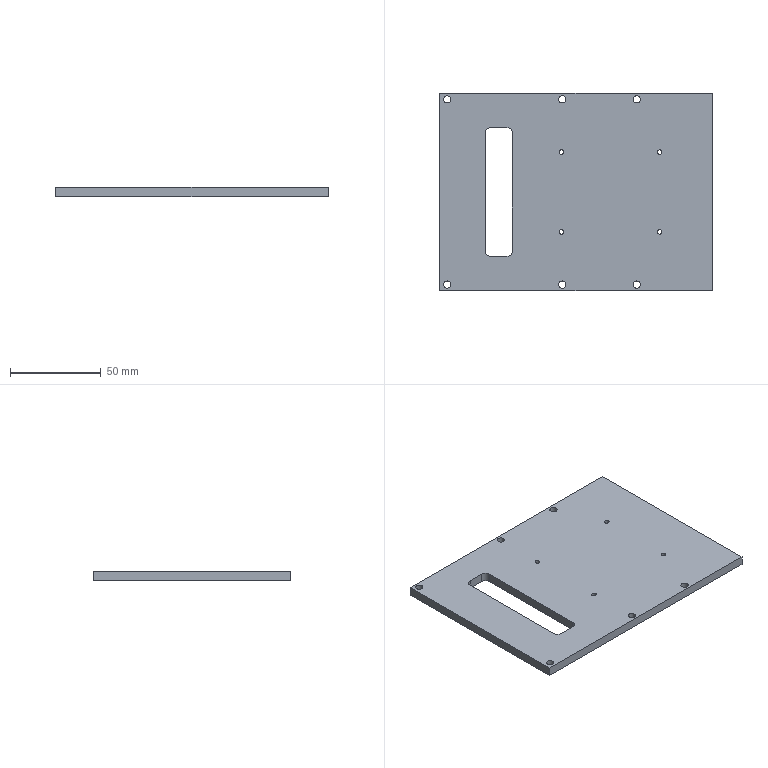Part | NX | 1 solid | 24 faces | box 150 x 108.5 x 5 mm | volume 75613 mm3 | cylinder 14 | plane 10 | commonest cylinder face diameters 4 x6 2.5 x4 6 x4
STEP:
#1=CARTESIAN_POINT('',(-38.,35.5,0.));
#2=VERTEX_POINT('',#1);
#3=CARTESIAN_POINT('',(-47.,35.5,0.));
#4=VERTEX_POINT('',#3);
#5=CARTESIAN_POINT('',(-38.,35.5,0.));
#6=DIRECTION('',(-1.,0.,0.));
#7=VECTOR('',#6,1000.);
#8=LINE('',#5,#7);
#9=EDGE_CURVE('',#2,#4,#8,.T.);
#10=ORIENTED_EDGE('',*,*,#9,.T.);
#11=CARTESIAN_POINT('',(-47.,35.5,-5.));
#12=VERTEX_POINT('',#11);
#13=CARTESIAN_POINT('',(-47.,35.5,-5.));
#14=DIRECTION('',(0.,0.,1.));
#15=VECTOR('',#14,1000.);
#16=LINE('',#13,#15);
#17=EDGE_CURVE('',#12,#4,#16,.T.);
#18=ORIENTED_EDGE('',*,*,#17,.F.);
#19=CARTESIAN_POINT('',(-38.,35.5,-5.));
#20=VERTEX_POINT('',#19);
#21=CARTESIAN_POINT('',(-38.,35.5,-5.));
#22=DIRECTION('',(-1.,0.,0.));
#23=VECTOR('',#22,1000.);
#24=LINE('',#21,#23);
#25=EDGE_CURVE('',#20,#12,#24,.T.);
#26=ORIENTED_EDGE('',*,*,#25,.F.);
#27=CARTESIAN_POINT('',(-38.,35.5,-5.));
#28=DIRECTION('',(0.,0.,1.));
#29=VECTOR('',#28,1000.);
#30=LINE('',#27,#29);
#31=EDGE_CURVE('',#20,#2,#30,.T.);
#32=ORIENTED_EDGE('',*,*,#31,.T.);
#33=EDGE_LOOP('',(#10,#18,#26,#32));
#34=FACE_BOUND('',#33,.T.);
#35=CARTESIAN_POINT('',(-38.,35.5,-5.));
#36=DIRECTION('',(0.,1.,0.));
#37=DIRECTION('',(-1.,0.,0.));
#38=AXIS2_PLACEMENT_3D('',#35,#36,#37);
#39=PLANE('',#38);
#40=ADVANCED_FACE('',(#34),#39,.F.);
#41=CARTESIAN_POINT('',(-35.,32.5,0.));
#42=VERTEX_POINT('',#41);
#43=CARTESIAN_POINT('',(-38.,32.5,0.));
#44=DIRECTION('',(0.,0.,1.));
#45=DIRECTION('',(0.,-1.,0.));
#46=AXIS2_PLACEMENT_3D('',#43,#44,#45);
#47=CIRCLE('',#46,3.);
#48=EDGE_CURVE('',#42,#2,#47,.T.);
#49=ORIENTED_EDGE('',*,*,#48,.T.);
#50=ORIENTED_EDGE('',*,*,#31,.F.);
#51=CARTESIAN_POINT('',(-35.,32.5,-5.));
#52=VERTEX_POINT('',#51);
#53=CARTESIAN_POINT('',(-38.,32.5,-5.));
#54=DIRECTION('',(0.,0.,1.));
#55=DIRECTION('',(0.,-1.,0.));
#56=AXIS2_PLACEMENT_3D('',#53,#54,#55);
#57=CIRCLE('',#56,3.);
#58=EDGE_CURVE('',#52,#20,#57,.T.);
#59=ORIENTED_EDGE('',*,*,#58,.F.);
#60=CARTESIAN_POINT('',(-35.,32.5,-5.));
#61=DIRECTION('',(0.,0.,1.));
#62=VECTOR('',#61,1000.);
#63=LINE('',#60,#62);
#64=EDGE_CURVE('',#52,#42,#63,.T.);
#65=ORIENTED_EDGE('',*,*,#64,.T.);
#66=EDGE_LOOP('',(#49,#50,#59,#65));
#67=FACE_BOUND('',#66,.T.);
#68=CARTESIAN_POINT('',(-38.,32.5,-5.));
#69=DIRECTION('',(0.,0.,1.));
#70=DIRECTION('',(0.,-1.,0.));
#71=AXIS2_PLACEMENT_3D('',#68,#69,#70);
#72=CYLINDRICAL_SURFACE('',#71,3.);
#73=ADVANCED_FACE('',(#67),#72,.F.);
#74=CARTESIAN_POINT('',(-35.,-32.5,0.));
#75=VERTEX_POINT('',#74);
#76=CARTESIAN_POINT('',(-35.,-32.5,0.));
#77=DIRECTION('',(0.,1.,0.));
#78=VECTOR('',#77,1000.);
#79=LINE('',#76,#78);
#80=EDGE_CURVE('',#75,#42,#79,.T.);
#81=ORIENTED_EDGE('',*,*,#80,.T.);
#82=ORIENTED_EDGE('',*,*,#64,.F.);
#83=CARTESIAN_POINT('',(-35.,-32.5,-5.));
#84=VERTEX_POINT('',#83);
#85=CARTESIAN_POINT('',(-35.,-32.5,-5.));
#86=DIRECTION('',(0.,1.,0.));
#87=VECTOR('',#86,1000.);
#88=LINE('',#85,#87);
#89=EDGE_CURVE('',#84,#52,#88,.T.);
#90=ORIENTED_EDGE('',*,*,#89,.F.);
#91=CARTESIAN_POINT('',(-35.,-32.5,-5.));
#92=DIRECTION('',(0.,0.,1.));
#93=VECTOR('',#92,1000.);
#94=LINE('',#91,#93);
#95=EDGE_CURVE('',#84,#75,#94,.T.);
#96=ORIENTED_EDGE('',*,*,#95,.T.);
#97=EDGE_LOOP('',(#81,#82,#90,#96));
#98=FACE_BOUND('',#97,.T.);
#99=CARTESIAN_POINT('',(-35.,-32.5,-5.));
#100=DIRECTION('',(1.,0.,0.));
#101=DIRECTION('',(0.,1.,0.));
#102=AXIS2_PLACEMENT_3D('',#99,#100,#101);
#103=PLANE('',#102);
#104=ADVANCED_FACE('',(#98),#103,.F.);
#105=CARTESIAN_POINT('',(-38.,-35.5,0.));
#106=VERTEX_POINT('',#105);
#107=CARTESIAN_POINT('',(-38.,-32.5,0.));
#108=DIRECTION('',(0.,0.,1.));
#109=DIRECTION('',(0.,-1.,0.));
#110=AXIS2_PLACEMENT_3D('',#107,#108,#109);
#111=CIRCLE('',#110,3.);
#112=EDGE_CURVE('',#106,#75,#111,.T.);
#113=ORIENTED_EDGE('',*,*,#112,.T.);
#114=ORIENTED_EDGE('',*,*,#95,.F.);
#115=CARTESIAN_POINT('',(-38.,-35.5,-5.));
#116=VERTEX_POINT('',#115);
#117=CARTESIAN_POINT('',(-38.,-32.5,-5.));
#118=DIRECTION('',(0.,0.,1.));
#119=DIRECTION('',(0.,-1.,0.));
#120=AXIS2_PLACEMENT_3D('',#117,#118,#119);
#121=CIRCLE('',#120,3.);
#122=EDGE_CURVE('',#116,#84,#121,.T.);
#123=ORIENTED_EDGE('',*,*,#122,.F.);
#124=CARTESIAN_POINT('',(-38.,-35.5,-5.));
#125=DIRECTION('',(0.,0.,1.));
#126=VECTOR('',#125,1000.);
#127=LINE('',#124,#126);
#128=EDGE_CURVE('',#116,#106,#127,.T.);
#129=ORIENTED_EDGE('',*,*,#128,.T.);
#130=EDGE_LOOP('',(#113,#114,#123,#129));
#131=FACE_BOUND('',#130,.T.);
#132=CARTESIAN_POINT('',(-38.,-32.5,-5.));
#133=DIRECTION('',(0.,0.,1.));
#134=DIRECTION('',(0.,-1.,0.));
#135=AXIS2_PLACEMENT_3D('',#132,#133,#134);
#136=CYLINDRICAL_SURFACE('',#135,3.);
#137=ADVANCED_FACE('',(#131),#136,.F.);
#138=CARTESIAN_POINT('',(-47.,-35.5,0.));
#139=VERTEX_POINT('',#138);
#140=CARTESIAN_POINT('',(-47.,-35.5,0.));
#141=DIRECTION('',(1.,0.,0.));
#142=VECTOR('',#141,1000.);
#143=LINE('',#140,#142);
#144=EDGE_CURVE('',#139,#106,#143,.T.);
#145=ORIENTED_EDGE('',*,*,#144,.T.);
#146=ORIENTED_EDGE('',*,*,#128,.F.);
#147=CARTESIAN_POINT('',(-47.,-35.5,-5.));
#148=VERTEX_POINT('',#147);
#149=CARTESIAN_POINT('',(-47.,-35.5,-5.));
#150=DIRECTION('',(1.,0.,0.));
#151=VECTOR('',#150,1000.);
#152=LINE('',#149,#151);
#153=EDGE_CURVE('',#148,#116,#152,.T.);
#154=ORIENTED_EDGE('',*,*,#153,.F.);
#155=CARTESIAN_POINT('',(-47.,-35.5,-5.));
#156=DIRECTION('',(0.,0.,1.));
#157=VECTOR('',#156,1000.);
#158=LINE('',#155,#157);
#159=EDGE_CURVE('',#148,#139,#158,.T.);
#160=ORIENTED_EDGE('',*,*,#159,.T.);
#161=EDGE_LOOP('',(#145,#146,#154,#160));
#162=FACE_BOUND('',#161,.T.);
#163=CARTESIAN_POINT('',(-47.,-35.5,-5.));
#164=DIRECTION('',(0.,-1.,0.));
#165=DIRECTION('',(0.,0.,-1.));
#166=AXIS2_PLACEMENT_3D('',#163,#164,#165);
#167=PLANE('',#166);
#168=ADVANCED_FACE('',(#162),#167,.F.);
#169=CARTESIAN_POINT('',(-50.,-32.5,0.));
#170=VERTEX_POINT('',#169);
#171=CARTESIAN_POINT('',(-47.,-32.5,0.));
#172=DIRECTION('',(0.,0.,1.));
#173=DIRECTION('',(0.,-1.,0.));
#174=AXIS2_PLACEMENT_3D('',#171,#172,#173);
#175=CIRCLE('',#174,3.);
#176=EDGE_CURVE('',#170,#139,#175,.T.);
#177=ORIENTED_EDGE('',*,*,#176,.T.);
#178=ORIENTED_EDGE('',*,*,#159,.F.);
#179=CARTESIAN_POINT('',(-50.,-32.5,-5.));
#180=VERTEX_POINT('',#179);
#181=CARTESIAN_POINT('',(-47.,-32.5,-5.));
#182=DIRECTION('',(0.,0.,1.));
#183=DIRECTION('',(0.,-1.,0.));
#184=AXIS2_PLACEMENT_3D('',#181,#182,#183);
#185=CIRCLE('',#184,3.);
#186=EDGE_CURVE('',#180,#148,#185,.T.);
#187=ORIENTED_EDGE('',*,*,#186,.F.);
#188=CARTESIAN_POINT('',(-50.,-32.5,-5.));
#189=DIRECTION('',(0.,0.,1.));
#190=VECTOR('',#189,1000.);
#191=LINE('',#188,#190);
#192=EDGE_CURVE('',#180,#170,#191,.T.);
#193=ORIENTED_EDGE('',*,*,#192,.T.);
#194=EDGE_LOOP('',(#177,#178,#187,#193));
#195=FACE_BOUND('',#194,.T.);
#196=CARTESIAN_POINT('',(-47.,-32.5,-5.));
#197=DIRECTION('',(0.,0.,1.));
#198=DIRECTION('',(0.,-1.,0.));
#199=AXIS2_PLACEMENT_3D('',#196,#197,#198);
#200=CYLINDRICAL_SURFACE('',#199,3.);
#201=ADVANCED_FACE('',(#195),#200,.F.);
#202=CARTESIAN_POINT('',(-50.,32.5,0.));
#203=VERTEX_POINT('',#202);
#204=CARTESIAN_POINT('',(-50.,32.5,0.));
#205=DIRECTION('',(0.,-1.,0.));
#206=VECTOR('',#205,1000.);
#207=LINE('',#204,#206);
#208=EDGE_CURVE('',#203,#170,#207,.T.);
#209=ORIENTED_EDGE('',*,*,#208,.T.);
#210=ORIENTED_EDGE('',*,*,#192,.F.);
#211=CARTESIAN_POINT('',(-50.,32.5,-5.));
#212=VERTEX_POINT('',#211);
#213=CARTESIAN_POINT('',(-50.,32.5,-5.));
#214=DIRECTION('',(0.,-1.,0.));
#215=VECTOR('',#214,1000.);
#216=LINE('',#213,#215);
#217=EDGE_CURVE('',#212,#180,#216,.T.);
#218=ORIENTED_EDGE('',*,*,#217,.F.);
#219=CARTESIAN_POINT('',(-50.,32.5,-5.));
#220=DIRECTION('',(0.,0.,1.));
#221=VECTOR('',#220,1000.);
#222=LINE('',#219,#221);
#223=EDGE_CURVE('',#212,#203,#222,.T.);
#224=ORIENTED_EDGE('',*,*,#223,.T.);
#225=EDGE_LOOP('',(#209,#210,#218,#224));
#226=FACE_BOUND('',#225,.T.);
#227=CARTESIAN_POINT('',(-50.,32.5,-5.));
#228=DIRECTION('',(-1.,0.,0.));
#229=DIRECTION('',(0.,0.,-1.));
#230=AXIS2_PLACEMENT_3D('',#227,#228,#229);
#231=PLANE('',#230);
#232=ADVANCED_FACE('',(#226),#231,.F.);
#233=CARTESIAN_POINT('',(75.,-54.25,0.));
#234=VERTEX_POINT('',#233);
#235=CARTESIAN_POINT('',(75.,54.25,0.));
#236=VERTEX_POINT('',#235);
#237=CARTESIAN_POINT('',(75.,-54.25,0.));
#238=DIRECTION('',(0.,1.,0.));
#239=VECTOR('',#238,1000.);
#240=LINE('',#237,#239);
#241=EDGE_CURVE('',#234,#236,#240,.T.);
#242=ORIENTED_EDGE('',*,*,#241,.F.);
#243=CARTESIAN_POINT('',(75.,-54.25,-5.));
#244=VERTEX_POINT('',#243);
#245=CARTESIAN_POINT('',(75.,-54.25,-5.));
#246=DIRECTION('',(0.,0.,1.));
#247=VECTOR('',#246,1000.);
#248=LINE('',#245,#247);
#249=EDGE_CURVE('',#244,#234,#248,.T.);
#250=ORIENTED_EDGE('',*,*,#249,.F.);
#251=CARTESIAN_POINT('',(75.,54.25,-5.));
#252=VERTEX_POINT('',#251);
#253=CARTESIAN_POINT('',(75.,-54.25,-5.));
#254=DIRECTION('',(0.,1.,0.));
#255=VECTOR('',#254,1000.);
#256=LINE('',#253,#255);
#257=EDGE_CURVE('',#244,#252,#256,.T.);
#258=ORIENTED_EDGE('',*,*,#257,.T.);
#259=CARTESIAN_POINT('',(75.,54.25,-5.));
#260=DIRECTION('',(0.,0.,1.));
#261=VECTOR('',#260,1000.);
#262=LINE('',#259,#261);
#263=EDGE_CURVE('',#252,#236,#262,.T.);
#264=ORIENTED_EDGE('',*,*,#263,.T.);
#265=EDGE_LOOP('',(#242,#250,#258,#264));
#266=FACE_BOUND('',#265,.T.);
#267=CARTESIAN_POINT('',(75.,-54.25,-5.));
#268=DIRECTION('',(1.,0.,0.));
#269=DIRECTION('',(0.,0.,1.));
#270=AXIS2_PLACEMENT_3D('',#267,#268,#269);
#271=PLANE('',#270);
#272=ADVANCED_FACE('',(#266),#271,.T.);
#273=CARTESIAN_POINT('',(-75.,54.25,0.));
#274=VERTEX_POINT('',#273);
#275=CARTESIAN_POINT('',(75.,54.25,0.));
#276=DIRECTION('',(-1.,0.,0.));
#277=VECTOR('',#276,1000.);
#278=LINE('',#275,#277);
#279=EDGE_CURVE('',#236,#274,#278,.T.);
#280=ORIENTED_EDGE('',*,*,#279,.F.);
#281=ORIENTED_EDGE('',*,*,#263,.F.);
#282=CARTESIAN_POINT('',(-75.,54.25,-5.));
#283=VERTEX_POINT('',#282);
#284=CARTESIAN_POINT('',(75.,54.25,-5.));
#285=DIRECTION('',(-1.,0.,0.));
#286=VECTOR('',#285,1000.);
#287=LINE('',#284,#286);
#288=EDGE_CURVE('',#252,#283,#287,.T.);
#289=ORIENTED_EDGE('',*,*,#288,.T.);
#290=CARTESIAN_POINT('',(-75.,54.25,-5.));
#291=DIRECTION('',(0.,0.,1.));
#292=VECTOR('',#291,1000.);
#293=LINE('',#290,#292);
#294=EDGE_CURVE('',#283,#274,#293,.T.);
#295=ORIENTED_EDGE('',*,*,#294,.T.);
#296=EDGE_LOOP('',(#280,#281,#289,#295));
#297=FACE_BOUND('',#296,.T.);
#298=CARTESIAN_POINT('',(75.,54.25,-5.));
#299=DIRECTION('',(0.,1.,0.));
#300=DIRECTION('',(0.,0.,1.));
#301=AXIS2_PLACEMENT_3D('',#298,#299,#300);
#302=PLANE('',#301);
#303=ADVANCED_FACE('',(#297),#302,.T.);
#304=CARTESIAN_POINT('',(-75.,-54.25,0.));
#305=VERTEX_POINT('',#304);
#306=CARTESIAN_POINT('',(-75.,54.25,0.));
#307=DIRECTION('',(0.,-1.,0.));
#308=VECTOR('',#307,1000.);
#309=LINE('',#306,#308);
#310=EDGE_CURVE('',#274,#305,#309,.T.);
#311=ORIENTED_EDGE('',*,*,#310,.F.);
#312=ORIENTED_EDGE('',*,*,#294,.F.);
#313=CARTESIAN_POINT('',(-75.,-54.25,-5.));
#314=VERTEX_POINT('',#313);
#315=CARTESIAN_POINT('',(-75.,54.25,-5.));
#316=DIRECTION('',(0.,-1.,0.));
#317=VECTOR('',#316,1000.);
#318=LINE('',#315,#317);
#319=EDGE_CURVE('',#283,#314,#318,.T.);
#320=ORIENTED_EDGE('',*,*,#319,.T.);
#321=CARTESIAN_POINT('',(-75.,-54.25,-5.));
#322=DIRECTION('',(0.,0.,1.));
#323=VECTOR('',#322,1000.);
#324=LINE('',#321,#323);
#325=EDGE_CURVE('',#314,#305,#324,.T.);
#326=ORIENTED_EDGE('',*,*,#325,.T.);
#327=EDGE_LOOP('',(#311,#312,#320,#326));
#328=FACE_BOUND('',#327,.T.);
#329=CARTESIAN_POINT('',(-75.,54.25,-5.));
#330=DIRECTION('',(-1.,0.,0.));
#331=DIRECTION('',(0.,0.,-1.));
#332=AXIS2_PLACEMENT_3D('',#329,#330,#331);
#333=PLANE('',#332);
#334=ADVANCED_FACE('',(#328),#333,.T.);
#335=CARTESIAN_POINT('',(-7.5,-53.,-5.));
#336=VERTEX_POINT('',#335);
#337=CARTESIAN_POINT('',(-7.5,-51.,-5.));
#338=DIRECTION('',(0.,0.,1.));
#339=DIRECTION('',(0.,-1.,0.));
#340=AXIS2_PLACEMENT_3D('',#337,#338,#339);
#341=CIRCLE('',#340,2.);
#342=EDGE_CURVE('',#336,#336,#341,.T.);
#343=ORIENTED_EDGE('',*,*,#342,.F.);
#344=EDGE_LOOP('',(#343));
#345=FACE_BOUND('',#344,.T.);
#346=CARTESIAN_POINT('',(-7.5,-53.,0.));
#347=VERTEX_POINT('',#346);
#348=CARTESIAN_POINT('',(-7.5,-51.,0.));
#349=DIRECTION('',(0.,0.,1.));
#350=DIRECTION('',(0.,-1.,0.));
#351=AXIS2_PLACEMENT_3D('',#348,#349,#350);
#352=CIRCLE('',#351,2.);
#353=EDGE_CURVE('',#347,#347,#352,.T.);
#354=ORIENTED_EDGE('',*,*,#353,.T.);
#355=EDGE_LOOP('',(#354));
#356=FACE_BOUND('',#355,.T.);
#357=CARTESIAN_POINT('',(-7.5,-51.,-5.));
#358=DIRECTION('',(0.,0.,1.));
#359=DIRECTION('',(0.,-1.,0.));
#360=AXIS2_PLACEMENT_3D('',#357,#358,#359);
#361=CYLINDRICAL_SURFACE('',#360,2.);
#362=ADVANCED_FACE('',(#345,#356),#361,.F.);
#363=CARTESIAN_POINT('',(-71.,-53.,-5.));
#364=VERTEX_POINT('',#363);
#365=CARTESIAN_POINT('',(-71.,-51.,-5.));
#366=DIRECTION('',(0.,0.,1.));
#367=DIRECTION('',(0.,-1.,0.));
#368=AXIS2_PLACEMENT_3D('',#365,#366,#367);
#369=CIRCLE('',#368,2.);
#370=EDGE_CURVE('',#364,#364,#369,.T.);
#371=ORIENTED_EDGE('',*,*,#370,.F.);
#372=EDGE_LOOP('',(#371));
#373=FACE_BOUND('',#372,.T.);
#374=CARTESIAN_POINT('',(-71.,-53.,0.));
#375=VERTEX_POINT('',#374);
#376=CARTESIAN_POINT('',(-71.,-51.,0.));
#377=DIRECTION('',(0.,0.,1.));
#378=DIRECTION('',(0.,-1.,0.));
#379=AXIS2_PLACEMENT_3D('',#376,#377,#378);
#380=CIRCLE('',#379,2.);
#381=EDGE_CURVE('',#375,#375,#380,.T.);
#382=ORIENTED_EDGE('',*,*,#381,.T.);
#383=EDGE_LOOP('',(#382));
#384=FACE_BOUND('',#383,.T.);
#385=CARTESIAN_POINT('',(-71.,-51.,-5.));
#386=DIRECTION('',(0.,0.,1.));
#387=DIRECTION('',(0.,-1.,0.));
#388=AXIS2_PLACEMENT_3D('',#385,#386,#387);
#389=CYLINDRICAL_SURFACE('',#388,2.);
#390=ADVANCED_FACE('',(#373,#384),#389,.F.);
#391=CARTESIAN_POINT('',(46.,-23.25,-5.));
#392=VERTEX_POINT('',#391);
#393=CARTESIAN_POINT('',(46.,-22.,-5.));
#394=DIRECTION('',(0.,0.,1.));
#395=DIRECTION('',(0.,-1.,0.));
#396=AXIS2_PLACEMENT_3D('',#393,#394,#395);
#397=CIRCLE('',#396,1.25);
#398=EDGE_CURVE('',#392,#392,#397,.T.);
#399=ORIENTED_EDGE('',*,*,#398,.F.);
#400=EDGE_LOOP('',(#399));
#401=FACE_BOUND('',#400,.T.);
#402=CARTESIAN_POINT('',(46.,-23.25,0.));
#403=VERTEX_POINT('',#402);
#404=CARTESIAN_POINT('',(46.,-22.,0.));
#405=DIRECTION('',(0.,0.,1.));
#406=DIRECTION('',(0.,-1.,0.));
#407=AXIS2_PLACEMENT_3D('',#404,#405,#406);
#408=CIRCLE('',#407,1.25);
#409=EDGE_CURVE('',#403,#403,#408,.T.);
#410=ORIENTED_EDGE('',*,*,#409,.T.);
#411=EDGE_LOOP('',(#410));
#412=FACE_BOUND('',#411,.T.);
#413=CARTESIAN_POINT('',(46.,-22.,-5.));
#414=DIRECTION('',(0.,0.,1.));
#415=DIRECTION('',(0.,-1.,0.));
#416=AXIS2_PLACEMENT_3D('',#413,#414,#415);
#417=CYLINDRICAL_SURFACE('',#416,1.25);
#418=ADVANCED_FACE('',(#401,#412),#417,.F.);
#419=CARTESIAN_POINT('',(-8.,-23.25,-5.));
#420=VERTEX_POINT('',#419);
#421=CARTESIAN_POINT('',(-8.,-22.,-5.));
#422=DIRECTION('',(0.,0.,1.));
#423=DIRECTION('',(0.,-1.,0.));
#424=AXIS2_PLACEMENT_3D('',#421,#422,#423);
#425=CIRCLE('',#424,1.25);
#426=EDGE_CURVE('',#420,#420,#425,.T.);
#427=ORIENTED_EDGE('',*,*,#426,.F.);
#428=EDGE_LOOP('',(#427));
#429=FACE_BOUND('',#428,.T.);
#430=CARTESIAN_POINT('',(-8.,-23.25,0.));
#431=VERTEX_POINT('',#430);
#432=CARTESIAN_POINT('',(-8.,-22.,0.));
#433=DIRECTION('',(0.,0.,1.));
#434=DIRECTION('',(0.,-1.,0.));
#435=AXIS2_PLACEMENT_3D('',#432,#433,#434);
#436=CIRCLE('',#435,1.25);
#437=EDGE_CURVE('',#431,#431,#436,.T.);
#438=ORIENTED_EDGE('',*,*,#437,.T.);
#439=EDGE_LOOP('',(#438));
#440=FACE_BOUND('',#439,.T.);
#441=CARTESIAN_POINT('',(-8.,-22.,-5.));
#442=DIRECTION('',(0.,0.,1.));
#443=DIRECTION('',(0.,-1.,0.));
#444=AXIS2_PLACEMENT_3D('',#441,#442,#443);
#445=CYLINDRICAL_SURFACE('',#444,1.25);
#446=ADVANCED_FACE('',(#429,#440),#445,.F.);
#447=CARTESIAN_POINT('',(46.,20.75,-5.));
#448=VERTEX_POINT('',#447);
#449=CARTESIAN_POINT('',(46.,22.,-5.));
#450=DIRECTION('',(0.,0.,1.));
#451=DIRECTION('',(0.,-1.,0.));
#452=AXIS2_PLACEMENT_3D('',#449,#450,#451);
#453=CIRCLE('',#452,1.25);
#454=EDGE_CURVE('',#448,#448,#453,.T.);
#455=ORIENTED_EDGE('',*,*,#454,.F.);
#456=EDGE_LOOP('',(#455));
#457=FACE_BOUND('',#456,.T.);
#458=CARTESIAN_POINT('',(46.,20.75,0.));
#459=VERTEX_POINT('',#458);
#460=CARTESIAN_POINT('',(46.,22.,0.));
#461=DIRECTION('',(0.,0.,1.));
#462=DIRECTION('',(0.,-1.,0.));
#463=AXIS2_PLACEMENT_3D('',#460,#461,#462);
#464=CIRCLE('',#463,1.25);
#465=EDGE_CURVE('',#459,#459,#464,.T.);
#466=ORIENTED_EDGE('',*,*,#465,.T.);
#467=EDGE_LOOP('',(#466));
#468=FACE_BOUND('',#467,.T.);
#469=CARTESIAN_POINT('',(46.,22.,-5.));
#470=DIRECTION('',(0.,0.,1.));
#471=DIRECTION('',(0.,-1.,0.));
#472=AXIS2_PLACEMENT_3D('',#469,#470,#471);
#473=CYLINDRICAL_SURFACE('',#472,1.25);
#474=ADVANCED_FACE('',(#457,#468),#473,.F.);
#475=CARTESIAN_POINT('',(-8.,20.75,-5.));
#476=VERTEX_POINT('',#475);
#477=CARTESIAN_POINT('',(-8.,22.,-5.));
#478=DIRECTION('',(0.,0.,1.));
#479=DIRECTION('',(0.,-1.,0.));
#480=AXIS2_PLACEMENT_3D('',#477,#478,#479);
#481=CIRCLE('',#480,1.25);
#482=EDGE_CURVE('',#476,#476,#481,.T.);
#483=ORIENTED_EDGE('',*,*,#482,.F.);
#484=EDGE_LOOP('',(#483));
#485=FACE_BOUND('',#484,.T.);
#486=CARTESIAN_POINT('',(-8.,20.75,0.));
#487=VERTEX_POINT('',#486);
#488=CARTESIAN_POINT('',(-8.,22.,0.));
#489=DIRECTION('',(0.,0.,1.));
#490=DIRECTION('',(0.,-1.,0.));
#491=AXIS2_PLACEMENT_3D('',#488,#489,#490);
#492=CIRCLE('',#491,1.25);
#493=EDGE_CURVE('',#487,#487,#492,.T.);
#494=ORIENTED_EDGE('',*,*,#493,.T.);
#495=EDGE_LOOP('',(#494));
#496=FACE_BOUND('',#495,.T.);
#497=CARTESIAN_POINT('',(-8.,22.,-5.));
#498=DIRECTION('',(0.,0.,1.));
#499=DIRECTION('',(0.,-1.,0.));
#500=AXIS2_PLACEMENT_3D('',#497,#498,#499);
#501=CYLINDRICAL_SURFACE('',#500,1.25);
#502=ADVANCED_FACE('',(#485,#496),#501,.F.);
#503=CARTESIAN_POINT('',(33.5,49.,-5.));
#504=VERTEX_POINT('',#503);
#505=CARTESIAN_POINT('',(33.5,51.,-5.));
#506=DIRECTION('',(0.,0.,1.));
#507=DIRECTION('',(0.,-1.,0.));
#508=AXIS2_PLACEMENT_3D('',#505,#506,#507);
#509=CIRCLE('',#508,2.);
#510=EDGE_CURVE('',#504,#504,#509,.T.);
#511=ORIENTED_EDGE('',*,*,#510,.F.);
#512=EDGE_LOOP('',(#511));
#513=FACE_BOUND('',#512,.T.);
#514=CARTESIAN_POINT('',(33.5,49.,0.));
#515=VERTEX_POINT('',#514);
#516=CARTESIAN_POINT('',(33.5,51.,0.));
#517=DIRECTION('',(0.,0.,1.));
#518=DIRECTION('',(0.,-1.,0.));
#519=AXIS2_PLACEMENT_3D('',#516,#517,#518);
#520=CIRCLE('',#519,2.);
#521=EDGE_CURVE('',#515,#515,#520,.T.);
#522=ORIENTED_EDGE('',*,*,#521,.T.);
#523=EDGE_LOOP('',(#522));
#524=FACE_BOUND('',#523,.T.);
#525=CARTESIAN_POINT('',(33.5,51.,-5.));
#526=DIRECTION('',(0.,0.,1.));
#527=DIRECTION('',(0.,-1.,0.));
#528=AXIS2_PLACEMENT_3D('',#525,#526,#527);
#529=CYLINDRICAL_SURFACE('',#528,2.);
#530=ADVANCED_FACE('',(#513,#524),#529,.F.);
#531=CARTESIAN_POINT('',(-7.5,49.,-5.));
#532=VERTEX_POINT('',#531);
#533=CARTESIAN_POINT('',(-7.5,51.,-5.));
#534=DIRECTION('',(0.,0.,1.));
#535=DIRECTION('',(0.,-1.,0.));
#536=AXIS2_PLACEMENT_3D('',#533,#534,#535);
#537=CIRCLE('',#536,2.);
#538=EDGE_CURVE('',#532,#532,#537,.T.);
#539=ORIENTED_EDGE('',*,*,#538,.F.);
#540=EDGE_LOOP('',(#539));
#541=FACE_BOUND('',#540,.T.);
#542=CARTESIAN_POINT('',(-7.5,49.,0.));
#543=VERTEX_POINT('',#542);
#544=CARTESIAN_POINT('',(-7.5,51.,0.));
#545=DIRECTION('',(0.,0.,1.));
#546=DIRECTION('',(0.,-1.,0.));
#547=AXIS2_PLACEMENT_3D('',#544,#545,#546);
#548=CIRCLE('',#547,2.);
#549=EDGE_CURVE('',#543,#543,#548,.T.);
#550=ORIENTED_EDGE('',*,*,#549,.T.);
#551=EDGE_LOOP('',(#550));
#552=FACE_BOUND('',#551,.T.);
#553=CARTESIAN_POINT('',(-7.5,51.,-5.));
#554=DIRECTION('',(0.,0.,1.));
#555=DIRECTION('',(0.,-1.,0.));
#556=AXIS2_PLACEMENT_3D('',#553,#554,#555);
#557=CYLINDRICAL_SURFACE('',#556,2.);
#558=ADVANCED_FACE('',(#541,#552),#557,.F.);
#559=CARTESIAN_POINT('',(-71.,49.,-5.));
#560=VERTEX_POINT('',#559);
#561=CARTESIAN_POINT('',(-71.,51.,-5.));
#562=DIRECTION('',(0.,0.,1.));
#563=DIRECTION('',(0.,-1.,0.));
#564=AXIS2_PLACEMENT_3D('',#561,#562,#563);
#565=CIRCLE('',#564,2.);
#566=EDGE_CURVE('',#560,#560,#565,.T.);
#567=ORIENTED_EDGE('',*,*,#566,.F.);
#568=EDGE_LOOP('',(#567));
#569=FACE_BOUND('',#568,.T.);
#570=CARTESIAN_POINT('',(-71.,49.,0.));
#571=VERTEX_POINT('',#570);
#572=CARTESIAN_POINT('',(-71.,51.,0.));
#573=DIRECTION('',(0.,0.,1.));
#574=DIRECTION('',(0.,-1.,0.));
#575=AXIS2_PLACEMENT_3D('',#572,#573,#574);
#576=CIRCLE('',#575,2.);
#577=EDGE_CURVE('',#571,#571,#576,.T.);
#578=ORIENTED_EDGE('',*,*,#577,.T.);
#579=EDGE_LOOP('',(#578));
#580=FACE_BOUND('',#579,.T.);
#581=CARTESIAN_POINT('',(-71.,51.,-5.));
#582=DIRECTION('',(0.,0.,1.));
#583=DIRECTION('',(0.,-1.,0.));
#584=AXIS2_PLACEMENT_3D('',#581,#582,#583);
#585=CYLINDRICAL_SURFACE('',#584,2.);
#586=ADVANCED_FACE('',(#569,#580),#585,.F.);
#587=CARTESIAN_POINT('',(-47.,32.5,0.));
#588=DIRECTION('',(0.,0.,1.));
#589=DIRECTION('',(0.,-1.,0.));
#590=AXIS2_PLACEMENT_3D('',#587,#588,#589);
#591=CIRCLE('',#590,3.);
#592=EDGE_CURVE('',#4,#203,#591,.T.);
#593=ORIENTED_EDGE('',*,*,#592,.T.);
#594=ORIENTED_EDGE('',*,*,#223,.F.);
#595=CARTESIAN_POINT('',(-47.,32.5,-5.));
#596=DIRECTION('',(0.,0.,1.));
#597=DIRECTION('',(0.,-1.,0.));
#598=AXIS2_PLACEMENT_3D('',#595,#596,#597);
#599=CIRCLE('',#598,3.);
#600=EDGE_CURVE('',#12,#212,#599,.T.);
#601=ORIENTED_EDGE('',*,*,#600,.F.);
#602=ORIENTED_EDGE('',*,*,#17,.T.);
#603=EDGE_LOOP('',(#593,#594,#601,#602));
#604=FACE_BOUND('',#603,.T.);
#605=CARTESIAN_POINT('',(-47.,32.5,-5.));
#606=DIRECTION('',(0.,0.,1.));
#607=DIRECTION('',(0.,-1.,0.));
#608=AXIS2_PLACEMENT_3D('',#605,#606,#607);
#609=CYLINDRICAL_SURFACE('',#608,3.);
#610=ADVANCED_FACE('',(#604),#609,.F.);
#611=CARTESIAN_POINT('',(-75.,-54.25,0.));
#612=DIRECTION('',(1.,0.,0.));
#613=VECTOR('',#612,1000.);
#614=LINE('',#611,#613);
#615=EDGE_CURVE('',#305,#234,#614,.T.);
#616=ORIENTED_EDGE('',*,*,#615,.F.);
#617=ORIENTED_EDGE('',*,*,#325,.F.);
#618=CARTESIAN_POINT('',(-75.,-54.25,-5.));
#619=DIRECTION('',(1.,0.,0.));
#620=VECTOR('',#619,1000.);
#621=LINE('',#618,#620);
#622=EDGE_CURVE('',#314,#244,#621,.T.);
#623=ORIENTED_EDGE('',*,*,#622,.T.);
#624=ORIENTED_EDGE('',*,*,#249,.T.);
#625=EDGE_LOOP('',(#616,#617,#623,#624));
#626=FACE_BOUND('',#625,.T.);
#627=CARTESIAN_POINT('',(-75.,-54.25,-5.));
#628=DIRECTION('',(0.,-1.,0.));
#629=DIRECTION('',(0.,0.,-1.));
#630=AXIS2_PLACEMENT_3D('',#627,#628,#629);
#631=PLANE('',#630);
#632=ADVANCED_FACE('',(#626),#631,.T.);
#633=CARTESIAN_POINT('',(33.5,-53.,-5.));
#634=VERTEX_POINT('',#633);
#635=CARTESIAN_POINT('',(33.5,-51.,-5.));
#636=DIRECTION('',(0.,0.,1.));
#637=DIRECTION('',(0.,-1.,0.));
#638=AXIS2_PLACEMENT_3D('',#635,#636,#637);
#639=CIRCLE('',#638,2.);
#640=EDGE_CURVE('',#634,#634,#639,.T.);
#641=ORIENTED_EDGE('',*,*,#640,.F.);
#642=EDGE_LOOP('',(#641));
#643=FACE_BOUND('',#642,.T.);
#644=CARTESIAN_POINT('',(33.5,-53.,0.));
#645=VERTEX_POINT('',#644);
#646=CARTESIAN_POINT('',(33.5,-51.,0.));
#647=DIRECTION('',(0.,0.,1.));
#648=DIRECTION('',(0.,-1.,0.));
#649=AXIS2_PLACEMENT_3D('',#646,#647,#648);
#650=CIRCLE('',#649,2.);
#651=EDGE_CURVE('',#645,#645,#650,.T.);
#652=ORIENTED_EDGE('',*,*,#651,.T.);
#653=EDGE_LOOP('',(#652));
#654=FACE_BOUND('',#653,.T.);
#655=CARTESIAN_POINT('',(33.5,-51.,-5.));
#656=DIRECTION('',(0.,0.,1.));
#657=DIRECTION('',(0.,-1.,0.));
#658=AXIS2_PLACEMENT_3D('',#655,#656,#657);
#659=CYLINDRICAL_SURFACE('',#658,2.);
#660=ADVANCED_FACE('',(#643,#654),#659,.F.);
#661=ORIENTED_EDGE('',*,*,#257,.F.);
#662=ORIENTED_EDGE('',*,*,#622,.F.);
#663=ORIENTED_EDGE('',*,*,#319,.F.);
#664=ORIENTED_EDGE('',*,*,#288,.F.);
#665=EDGE_LOOP('',(#661,#662,#663,#664));
#666=FACE_BOUND('',#665,.T.);
#667=ORIENTED_EDGE('',*,*,#25,.T.);
#668=ORIENTED_EDGE('',*,*,#600,.T.);
#669=ORIENTED_EDGE('',*,*,#217,.T.);
#670=ORIENTED_EDGE('',*,*,#186,.T.);
#671=ORIENTED_EDGE('',*,*,#153,.T.);
#672=ORIENTED_EDGE('',*,*,#122,.T.);
#673=ORIENTED_EDGE('',*,*,#89,.T.);
#674=ORIENTED_EDGE('',*,*,#58,.T.);
#675=EDGE_LOOP('',(#667,#668,#669,#670,#671,#672,#673,#674));
#676=FACE_BOUND('',#675,.T.);
#677=ORIENTED_EDGE('',*,*,#566,.T.);
#678=EDGE_LOOP('',(#677));
#679=FACE_BOUND('',#678,.T.);
#680=ORIENTED_EDGE('',*,*,#538,.T.);
#681=EDGE_LOOP('',(#680));
#682=FACE_BOUND('',#681,.T.);
#683=ORIENTED_EDGE('',*,*,#510,.T.);
#684=EDGE_LOOP('',(#683));
#685=FACE_BOUND('',#684,.T.);
#686=ORIENTED_EDGE('',*,*,#482,.T.);
#687=EDGE_LOOP('',(#686));
#688=FACE_BOUND('',#687,.T.);
#689=ORIENTED_EDGE('',*,*,#454,.T.);
#690=EDGE_LOOP('',(#689));
#691=FACE_BOUND('',#690,.T.);
#692=ORIENTED_EDGE('',*,*,#426,.T.);
#693=EDGE_LOOP('',(#692));
#694=FACE_BOUND('',#693,.T.);
#695=ORIENTED_EDGE('',*,*,#398,.T.);
#696=EDGE_LOOP('',(#695));
#697=FACE_BOUND('',#696,.T.);
#698=ORIENTED_EDGE('',*,*,#370,.T.);
#699=EDGE_LOOP('',(#698));
#700=FACE_BOUND('',#699,.T.);
#701=ORIENTED_EDGE('',*,*,#342,.T.);
#702=EDGE_LOOP('',(#701));
#703=FACE_BOUND('',#702,.T.);
#704=ORIENTED_EDGE('',*,*,#640,.T.);
#705=EDGE_LOOP('',(#704));
#706=FACE_BOUND('',#705,.T.);
#707=CARTESIAN_POINT('',(-38.,32.5,-5.));
#708=DIRECTION('',(0.,0.,1.));
#709=DIRECTION('',(0.,-1.,0.));
#710=AXIS2_PLACEMENT_3D('',#707,#708,#709);
#711=PLANE('',#710);
#712=ADVANCED_FACE('',(#666,#676,#679,#682,#685,#688,#691,#694,#697,#700,#703,#706),#711,.F.);
#713=ORIENTED_EDGE('',*,*,#241,.T.);
#714=ORIENTED_EDGE('',*,*,#279,.T.);
#715=ORIENTED_EDGE('',*,*,#310,.T.);
#716=ORIENTED_EDGE('',*,*,#615,.T.);
#717=EDGE_LOOP('',(#713,#714,#715,#716));
#718=FACE_BOUND('',#717,.T.);
#719=ORIENTED_EDGE('',*,*,#9,.F.);
#720=ORIENTED_EDGE('',*,*,#48,.F.);
#721=ORIENTED_EDGE('',*,*,#80,.F.);
#722=ORIENTED_EDGE('',*,*,#112,.F.);
#723=ORIENTED_EDGE('',*,*,#144,.F.);
#724=ORIENTED_EDGE('',*,*,#176,.F.);
#725=ORIENTED_EDGE('',*,*,#208,.F.);
#726=ORIENTED_EDGE('',*,*,#592,.F.);
#727=EDGE_LOOP('',(#719,#720,#721,#722,#723,#724,#725,#726));
#728=FACE_BOUND('',#727,.T.);
#729=ORIENTED_EDGE('',*,*,#577,.F.);
#730=EDGE_LOOP('',(#729));
#731=FACE_BOUND('',#730,.T.);
#732=ORIENTED_EDGE('',*,*,#549,.F.);
#733=EDGE_LOOP('',(#732));
#734=FACE_BOUND('',#733,.T.);
#735=ORIENTED_EDGE('',*,*,#521,.F.);
#736=EDGE_LOOP('',(#735));
#737=FACE_BOUND('',#736,.T.);
#738=ORIENTED_EDGE('',*,*,#493,.F.);
#739=EDGE_LOOP('',(#738));
#740=FACE_BOUND('',#739,.T.);
#741=ORIENTED_EDGE('',*,*,#465,.F.);
#742=EDGE_LOOP('',(#741));
#743=FACE_BOUND('',#742,.T.);
#744=ORIENTED_EDGE('',*,*,#437,.F.);
#745=EDGE_LOOP('',(#744));
#746=FACE_BOUND('',#745,.T.);
#747=ORIENTED_EDGE('',*,*,#409,.F.);
#748=EDGE_LOOP('',(#747));
#749=FACE_BOUND('',#748,.T.);
#750=ORIENTED_EDGE('',*,*,#381,.F.);
#751=EDGE_LOOP('',(#750));
#752=FACE_BOUND('',#751,.T.);
#753=ORIENTED_EDGE('',*,*,#353,.F.);
#754=EDGE_LOOP('',(#753));
#755=FACE_BOUND('',#754,.T.);
#756=ORIENTED_EDGE('',*,*,#651,.F.);
#757=EDGE_LOOP('',(#756));
#758=FACE_BOUND('',#757,.T.);
#759=CARTESIAN_POINT('',(-38.,32.5,0.));
#760=DIRECTION('',(0.,0.,1.));
#761=DIRECTION('',(0.,-1.,0.));
#762=AXIS2_PLACEMENT_3D('',#759,#760,#761);
#763=PLANE('',#762);
#764=ADVANCED_FACE('',(#718,#728,#731,#734,#737,#740,#743,#746,#749,#752,#755,#758),#763,.T.);
#765=CLOSED_SHELL('',(#40,#73,#104,#137,#168,#201,#232,#272,#303,#334,#362,#390,#418,#446,#474,#502,#530,#558,#586,#610,#632,#660,#712,#764));
#766=MANIFOLD_SOLID_BREP('',#765);
#767=(LENGTH_UNIT()NAMED_UNIT(*)SI_UNIT(.MILLI.,.METRE.));
#768=UNCERTAINTY_MEASURE_WITH_UNIT(LENGTH_MEASURE(0.00001),#767,'','');
#769=(NAMED_UNIT(*)PLANE_ANGLE_UNIT()SI_UNIT($,.RADIAN.));
#770=(NAMED_UNIT(*)SI_UNIT($,.STERADIAN.)SOLID_ANGLE_UNIT());
#771=(GEOMETRIC_REPRESENTATION_CONTEXT(3)GLOBAL_UNCERTAINTY_ASSIGNED_CONTEXT((#768))GLOBAL_UNIT_ASSIGNED_CONTEXT((#767,#769,#770))REPRESENTATION_CONTEXT('',''));
#772=ADVANCED_BREP_SHAPE_REPRESENTATION('',(#766),#771);